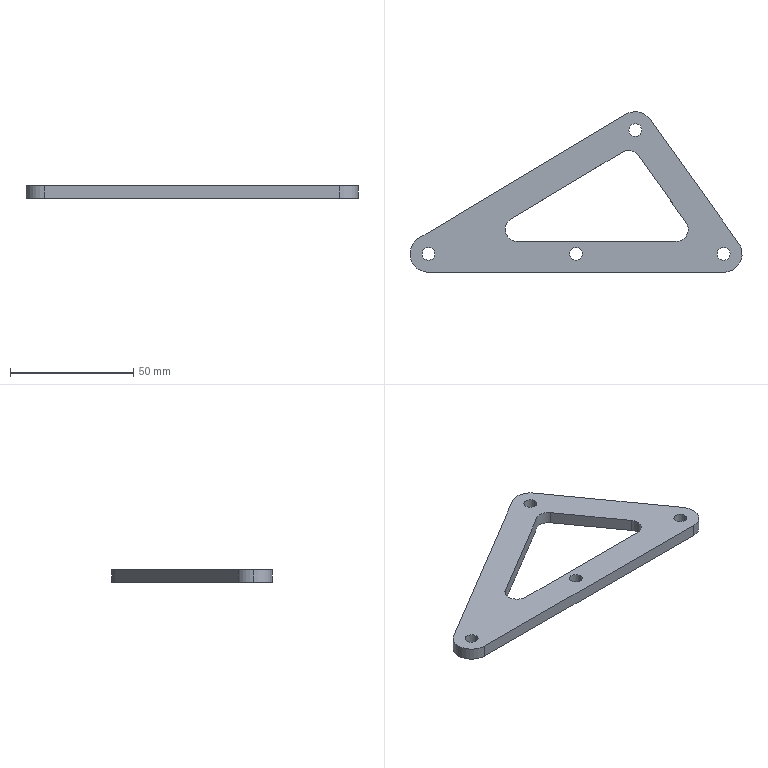Part | SolidWorks | features Extrusion 1 | 1 solid | 24 faces | box 135 x 65.308 x 5 mm | volume 17553 mm3 | cylinder 16 | plane 8 | commonest cylinder face diameters 5.2 x8 10 x4 15 x4
STEP:
#1=CARTESIAN_POINT('',(-50.457,-36.017,5.));
#2=VERTEX_POINT('',#1);
#3=CARTESIAN_POINT('',(-52.89,-40.308,5.));
#4=VERTEX_POINT('',#3);
#5=CARTESIAN_POINT('',(-47.89,-40.308,5.));
#6=DIRECTION('',(0.,0.,1.));
#7=DIRECTION('',(-1.,0.,0.));
#8=AXIS2_PLACEMENT_3D('',#5,#6,#7);
#9=CIRCLE('',#8,5.);
#10=EDGE_CURVE('',#2,#4,#9,.T.);
#11=ORIENTED_EDGE('',*,*,#10,.T.);
#12=CARTESIAN_POINT('',(-52.89,-40.308,0.));
#13=VERTEX_POINT('',#12);
#14=CARTESIAN_POINT('',(-52.89,-40.308,5.));
#15=DIRECTION('',(0.,0.,-1.));
#16=VECTOR('',#15,1000.);
#17=LINE('',#14,#16);
#18=EDGE_CURVE('',#4,#13,#17,.T.);
#19=ORIENTED_EDGE('',*,*,#18,.T.);
#20=CARTESIAN_POINT('',(-50.457,-36.017,0.));
#21=VERTEX_POINT('',#20);
#22=CARTESIAN_POINT('',(-47.89,-40.308,0.));
#23=DIRECTION('',(0.,0.,1.));
#24=DIRECTION('',(-1.,0.,0.));
#25=AXIS2_PLACEMENT_3D('',#22,#23,#24);
#26=CIRCLE('',#25,5.);
#27=EDGE_CURVE('',#21,#13,#26,.T.);
#28=ORIENTED_EDGE('',*,*,#27,.F.);
#29=CARTESIAN_POINT('',(-50.457,-36.017,5.));
#30=DIRECTION('',(0.,0.,-1.));
#31=VECTOR('',#30,1000.);
#32=LINE('',#29,#31);
#33=EDGE_CURVE('',#2,#21,#32,.T.);
#34=ORIENTED_EDGE('',*,*,#33,.F.);
#35=EDGE_LOOP('',(#11,#19,#28,#34));
#36=FACE_OUTER_BOUND('',#35,.T.);
#37=CARTESIAN_POINT('',(-47.89,-40.308,5.));
#38=DIRECTION('',(0.,0.,-1.));
#39=DIRECTION('',(-1.,0.,0.));
#40=AXIS2_PLACEMENT_3D('',#37,#38,#39);
#41=CYLINDRICAL_SURFACE('',#40,5.);
#42=ADVANCED_FACE('',(#36),#41,.F.);
#43=CARTESIAN_POINT('',(-2.6,0.,5.));
#44=VERTEX_POINT('',#43);
#45=CARTESIAN_POINT('',(2.6,0.,5.));
#46=VERTEX_POINT('',#45);
#47=CARTESIAN_POINT('',(0.,0.,5.));
#48=DIRECTION('',(0.,0.,1.));
#49=DIRECTION('',(1.,0.,0.));
#50=AXIS2_PLACEMENT_3D('',#47,#48,#49);
#51=CIRCLE('',#50,2.6);
#52=EDGE_CURVE('',#44,#46,#51,.T.);
#53=ORIENTED_EDGE('',*,*,#52,.T.);
#54=CARTESIAN_POINT('',(2.6,0.,0.));
#55=VERTEX_POINT('',#54);
#56=CARTESIAN_POINT('',(2.6,0.,5.));
#57=DIRECTION('',(0.,0.,-1.));
#58=VECTOR('',#57,1000.);
#59=LINE('',#56,#58);
#60=EDGE_CURVE('',#46,#55,#59,.T.);
#61=ORIENTED_EDGE('',*,*,#60,.T.);
#62=CARTESIAN_POINT('',(-2.6,0.,0.));
#63=VERTEX_POINT('',#62);
#64=CARTESIAN_POINT('',(0.,0.,0.));
#65=DIRECTION('',(0.,0.,1.));
#66=DIRECTION('',(1.,0.,0.));
#67=AXIS2_PLACEMENT_3D('',#64,#65,#66);
#68=CIRCLE('',#67,2.6);
#69=EDGE_CURVE('',#63,#55,#68,.T.);
#70=ORIENTED_EDGE('',*,*,#69,.F.);
#71=CARTESIAN_POINT('',(-2.6,0.,5.));
#72=DIRECTION('',(0.,0.,-1.));
#73=VECTOR('',#72,1000.);
#74=LINE('',#71,#73);
#75=EDGE_CURVE('',#44,#63,#74,.T.);
#76=ORIENTED_EDGE('',*,*,#75,.F.);
#77=EDGE_LOOP('',(#53,#61,#70,#76));
#78=FACE_OUTER_BOUND('',#77,.T.);
#79=CARTESIAN_POINT('',(0.,0.,5.));
#80=DIRECTION('',(0.,0.,-1.));
#81=DIRECTION('',(-1.,0.,0.));
#82=AXIS2_PLACEMENT_3D('',#79,#80,#81);
#83=CYLINDRICAL_SURFACE('',#82,2.6);
#84=ADVANCED_FACE('',(#78),#83,.F.);
#85=CARTESIAN_POINT('',(-86.68,-50.308,5.));
#86=VERTEX_POINT('',#85);
#87=CARTESIAN_POINT('',(-81.48,-50.308,5.));
#88=VERTEX_POINT('',#87);
#89=CARTESIAN_POINT('',(-84.08,-50.308,5.));
#90=DIRECTION('',(0.,0.,1.));
#91=DIRECTION('',(1.,0.,0.));
#92=AXIS2_PLACEMENT_3D('',#89,#90,#91);
#93=CIRCLE('',#92,2.6);
#94=EDGE_CURVE('',#86,#88,#93,.T.);
#95=ORIENTED_EDGE('',*,*,#94,.T.);
#96=CARTESIAN_POINT('',(-81.48,-50.308,0.));
#97=VERTEX_POINT('',#96);
#98=CARTESIAN_POINT('',(-81.48,-50.308,5.));
#99=DIRECTION('',(0.,0.,-1.));
#100=VECTOR('',#99,1000.);
#101=LINE('',#98,#100);
#102=EDGE_CURVE('',#88,#97,#101,.T.);
#103=ORIENTED_EDGE('',*,*,#102,.T.);
#104=CARTESIAN_POINT('',(-86.68,-50.308,0.));
#105=VERTEX_POINT('',#104);
#106=CARTESIAN_POINT('',(-84.08,-50.308,0.));
#107=DIRECTION('',(0.,0.,1.));
#108=DIRECTION('',(1.,0.,0.));
#109=AXIS2_PLACEMENT_3D('',#106,#107,#108);
#110=CIRCLE('',#109,2.6);
#111=EDGE_CURVE('',#105,#97,#110,.T.);
#112=ORIENTED_EDGE('',*,*,#111,.F.);
#113=CARTESIAN_POINT('',(-86.68,-50.308,5.));
#114=DIRECTION('',(0.,0.,-1.));
#115=VECTOR('',#114,1000.);
#116=LINE('',#113,#115);
#117=EDGE_CURVE('',#86,#105,#116,.T.);
#118=ORIENTED_EDGE('',*,*,#117,.F.);
#119=EDGE_LOOP('',(#95,#103,#112,#118));
#120=FACE_OUTER_BOUND('',#119,.T.);
#121=CARTESIAN_POINT('',(-84.08,-50.308,5.));
#122=DIRECTION('',(0.,0.,-1.));
#123=DIRECTION('',(-1.,0.,0.));
#124=AXIS2_PLACEMENT_3D('',#121,#122,#123);
#125=CYLINDRICAL_SURFACE('',#124,2.6);
#126=ADVANCED_FACE('',(#120),#125,.F.);
#127=CARTESIAN_POINT('',(33.32,-50.308,5.));
#128=VERTEX_POINT('',#127);
#129=CARTESIAN_POINT('',(38.52,-50.308,5.));
#130=VERTEX_POINT('',#129);
#131=CARTESIAN_POINT('',(35.92,-50.308,5.));
#132=DIRECTION('',(0.,0.,1.));
#133=DIRECTION('',(1.,0.,0.));
#134=AXIS2_PLACEMENT_3D('',#131,#132,#133);
#135=CIRCLE('',#134,2.6);
#136=EDGE_CURVE('',#128,#130,#135,.T.);
#137=ORIENTED_EDGE('',*,*,#136,.T.);
#138=CARTESIAN_POINT('',(38.52,-50.308,0.));
#139=VERTEX_POINT('',#138);
#140=CARTESIAN_POINT('',(38.52,-50.308,5.));
#141=DIRECTION('',(0.,0.,-1.));
#142=VECTOR('',#141,1000.);
#143=LINE('',#140,#142);
#144=EDGE_CURVE('',#130,#139,#143,.T.);
#145=ORIENTED_EDGE('',*,*,#144,.T.);
#146=CARTESIAN_POINT('',(33.32,-50.308,0.));
#147=VERTEX_POINT('',#146);
#148=CARTESIAN_POINT('',(35.92,-50.308,0.));
#149=DIRECTION('',(0.,0.,1.));
#150=DIRECTION('',(1.,0.,0.));
#151=AXIS2_PLACEMENT_3D('',#148,#149,#150);
#152=CIRCLE('',#151,2.6);
#153=EDGE_CURVE('',#147,#139,#152,.T.);
#154=ORIENTED_EDGE('',*,*,#153,.F.);
#155=CARTESIAN_POINT('',(33.32,-50.308,5.));
#156=DIRECTION('',(0.,0.,-1.));
#157=VECTOR('',#156,1000.);
#158=LINE('',#155,#157);
#159=EDGE_CURVE('',#128,#147,#158,.T.);
#160=ORIENTED_EDGE('',*,*,#159,.F.);
#161=EDGE_LOOP('',(#137,#145,#154,#160));
#162=FACE_OUTER_BOUND('',#161,.T.);
#163=CARTESIAN_POINT('',(35.92,-50.308,5.));
#164=DIRECTION('',(0.,0.,-1.));
#165=DIRECTION('',(-1.,0.,0.));
#166=AXIS2_PLACEMENT_3D('',#163,#164,#165);
#167=CYLINDRICAL_SURFACE('',#166,2.6);
#168=ADVANCED_FACE('',(#162),#167,.F.);
#169=CARTESIAN_POINT('',(-26.68,-50.308,5.));
#170=VERTEX_POINT('',#169);
#171=CARTESIAN_POINT('',(-21.48,-50.308,5.));
#172=VERTEX_POINT('',#171);
#173=CARTESIAN_POINT('',(-24.08,-50.308,5.));
#174=DIRECTION('',(0.,0.,1.));
#175=DIRECTION('',(1.,0.,0.));
#176=AXIS2_PLACEMENT_3D('',#173,#174,#175);
#177=CIRCLE('',#176,2.6);
#178=EDGE_CURVE('',#170,#172,#177,.T.);
#179=ORIENTED_EDGE('',*,*,#178,.T.);
#180=CARTESIAN_POINT('',(-21.48,-50.308,0.));
#181=VERTEX_POINT('',#180);
#182=CARTESIAN_POINT('',(-21.48,-50.308,5.));
#183=DIRECTION('',(0.,0.,-1.));
#184=VECTOR('',#183,1000.);
#185=LINE('',#182,#184);
#186=EDGE_CURVE('',#172,#181,#185,.T.);
#187=ORIENTED_EDGE('',*,*,#186,.T.);
#188=CARTESIAN_POINT('',(-26.68,-50.308,0.));
#189=VERTEX_POINT('',#188);
#190=CARTESIAN_POINT('',(-24.08,-50.308,0.));
#191=DIRECTION('',(0.,0.,1.));
#192=DIRECTION('',(1.,0.,0.));
#193=AXIS2_PLACEMENT_3D('',#190,#191,#192);
#194=CIRCLE('',#193,2.6);
#195=EDGE_CURVE('',#189,#181,#194,.T.);
#196=ORIENTED_EDGE('',*,*,#195,.F.);
#197=CARTESIAN_POINT('',(-26.68,-50.308,5.));
#198=DIRECTION('',(0.,0.,-1.));
#199=VECTOR('',#198,1000.);
#200=LINE('',#197,#199);
#201=EDGE_CURVE('',#170,#189,#200,.T.);
#202=ORIENTED_EDGE('',*,*,#201,.F.);
#203=EDGE_LOOP('',(#179,#187,#196,#202));
#204=FACE_OUTER_BOUND('',#203,.T.);
#205=CARTESIAN_POINT('',(-24.08,-50.308,5.));
#206=DIRECTION('',(0.,0.,-1.));
#207=DIRECTION('',(-1.,0.,0.));
#208=AXIS2_PLACEMENT_3D('',#205,#206,#207);
#209=CYLINDRICAL_SURFACE('',#208,2.6);
#210=ADVANCED_FACE('',(#204),#209,.F.);
#211=CARTESIAN_POINT('',(-91.58,-50.308,5.));
#212=VERTEX_POINT('',#211);
#213=CARTESIAN_POINT('',(-84.08,-57.808,5.));
#214=VERTEX_POINT('',#213);
#215=CARTESIAN_POINT('',(-84.08,-50.308,5.));
#216=DIRECTION('',(0.,0.,1.));
#217=DIRECTION('',(1.,0.,0.));
#218=AXIS2_PLACEMENT_3D('',#215,#216,#217);
#219=CIRCLE('',#218,7.5);
#220=EDGE_CURVE('',#212,#214,#219,.T.);
#221=ORIENTED_EDGE('',*,*,#220,.F.);
#222=CARTESIAN_POINT('',(-91.58,-50.308,0.));
#223=VERTEX_POINT('',#222);
#224=CARTESIAN_POINT('',(-91.58,-50.308,5.));
#225=DIRECTION('',(0.,0.,-1.));
#226=VECTOR('',#225,1000.);
#227=LINE('',#224,#226);
#228=EDGE_CURVE('',#212,#223,#227,.T.);
#229=ORIENTED_EDGE('',*,*,#228,.T.);
#230=CARTESIAN_POINT('',(-84.08,-57.808,0.));
#231=VERTEX_POINT('',#230);
#232=CARTESIAN_POINT('',(-84.08,-50.308,0.));
#233=DIRECTION('',(0.,0.,1.));
#234=DIRECTION('',(1.,0.,0.));
#235=AXIS2_PLACEMENT_3D('',#232,#233,#234);
#236=CIRCLE('',#235,7.5);
#237=EDGE_CURVE('',#223,#231,#236,.T.);
#238=ORIENTED_EDGE('',*,*,#237,.T.);
#239=CARTESIAN_POINT('',(-84.08,-57.808,5.));
#240=DIRECTION('',(0.,0.,-1.));
#241=VECTOR('',#240,1000.);
#242=LINE('',#239,#241);
#243=EDGE_CURVE('',#214,#231,#242,.T.);
#244=ORIENTED_EDGE('',*,*,#243,.F.);
#245=EDGE_LOOP('',(#221,#229,#238,#244));
#246=FACE_OUTER_BOUND('',#245,.T.);
#247=CARTESIAN_POINT('',(-84.08,-50.308,5.));
#248=DIRECTION('',(0.,0.,-1.));
#249=DIRECTION('',(-1.,0.,0.));
#250=AXIS2_PLACEMENT_3D('',#247,#248,#249);
#251=CYLINDRICAL_SURFACE('',#250,7.5);
#252=ADVANCED_FACE('',(#246),#251,.T.);
#253=ORIENTED_EDGE('',*,*,#94,.F.);
#254=CARTESIAN_POINT('',(-84.08,-50.308,5.));
#255=DIRECTION('',(0.,0.,1.));
#256=DIRECTION('',(1.,0.,0.));
#257=AXIS2_PLACEMENT_3D('',#254,#255,#256);
#258=CIRCLE('',#257,2.6);
#259=EDGE_CURVE('',#88,#86,#258,.T.);
#260=ORIENTED_EDGE('',*,*,#259,.F.);
#261=EDGE_LOOP('',(#253,#260));
#262=FACE_BOUND('',#261,.T.);
#263=ORIENTED_EDGE('',*,*,#178,.F.);
#264=CARTESIAN_POINT('',(-24.08,-50.308,5.));
#265=DIRECTION('',(0.,0.,1.));
#266=DIRECTION('',(1.,0.,0.));
#267=AXIS2_PLACEMENT_3D('',#264,#265,#266);
#268=CIRCLE('',#267,2.6);
#269=EDGE_CURVE('',#172,#170,#268,.T.);
#270=ORIENTED_EDGE('',*,*,#269,.F.);
#271=EDGE_LOOP('',(#263,#270));
#272=FACE_BOUND('',#271,.T.);
#273=CARTESIAN_POINT('',(35.92,-57.808,5.));
#274=VERTEX_POINT('',#273);
#275=CARTESIAN_POINT('',(-24.08,-57.808,5.));
#276=DIRECTION('',(1.,0.,0.));
#277=VECTOR('',#276,1000.);
#278=LINE('',#275,#277);
#279=EDGE_CURVE('',#214,#274,#278,.T.);
#280=ORIENTED_EDGE('',*,*,#279,.T.);
#281=CARTESIAN_POINT('',(42.024,-45.949,5.));
#282=VERTEX_POINT('',#281);
#283=CARTESIAN_POINT('',(35.92,-50.308,5.));
#284=DIRECTION('',(0.,0.,1.));
#285=DIRECTION('',(1.,0.,0.));
#286=AXIS2_PLACEMENT_3D('',#283,#284,#285);
#287=CIRCLE('',#286,7.5);
#288=EDGE_CURVE('',#274,#282,#287,.T.);
#289=ORIENTED_EDGE('',*,*,#288,.T.);
#290=CARTESIAN_POINT('',(6.104,4.358,5.));
#291=VERTEX_POINT('',#290);
#292=CARTESIAN_POINT('',(42.024,-45.949,5.));
#293=DIRECTION('',(-0.5811,0.8138,0.));
#294=VECTOR('',#293,1000.);
#295=LINE('',#292,#294);
#296=EDGE_CURVE('',#282,#291,#295,.T.);
#297=ORIENTED_EDGE('',*,*,#296,.T.);
#298=CARTESIAN_POINT('',(-3.851,6.436,5.));
#299=VERTEX_POINT('',#298);
#300=CARTESIAN_POINT('',(0.,0.,5.));
#301=DIRECTION('',(0.,0.,1.));
#302=DIRECTION('',(1.,0.,0.));
#303=AXIS2_PLACEMENT_3D('',#300,#301,#302);
#304=CIRCLE('',#303,7.5);
#305=EDGE_CURVE('',#291,#299,#304,.T.);
#306=ORIENTED_EDGE('',*,*,#305,.T.);
#307=CARTESIAN_POINT('',(-87.93,-43.872,5.));
#308=VERTEX_POINT('',#307);
#309=CARTESIAN_POINT('',(-3.851,6.436,5.));
#310=DIRECTION('',(-0.8581,-0.5134,0.));
#311=VECTOR('',#310,1000.);
#312=LINE('',#309,#311);
#313=EDGE_CURVE('',#299,#308,#312,.T.);
#314=ORIENTED_EDGE('',*,*,#313,.T.);
#315=CARTESIAN_POINT('',(-84.08,-50.308,5.));
#316=DIRECTION('',(0.,0.,1.));
#317=DIRECTION('',(1.,0.,0.));
#318=AXIS2_PLACEMENT_3D('',#315,#316,#317);
#319=CIRCLE('',#318,7.5);
#320=EDGE_CURVE('',#308,#212,#319,.T.);
#321=ORIENTED_EDGE('',*,*,#320,.T.);
#322=ORIENTED_EDGE('',*,*,#220,.T.);
#323=EDGE_LOOP('',(#280,#289,#297,#306,#314,#321,#322));
#324=FACE_OUTER_BOUND('',#323,.T.);
#325=ORIENTED_EDGE('',*,*,#136,.F.);
#326=CARTESIAN_POINT('',(35.92,-50.308,5.));
#327=DIRECTION('',(0.,0.,1.));
#328=DIRECTION('',(1.,0.,0.));
#329=AXIS2_PLACEMENT_3D('',#326,#327,#328);
#330=CIRCLE('',#329,2.6);
#331=EDGE_CURVE('',#130,#128,#330,.T.);
#332=ORIENTED_EDGE('',*,*,#331,.F.);
#333=EDGE_LOOP('',(#325,#332));
#334=FACE_BOUND('',#333,.T.);
#335=ORIENTED_EDGE('',*,*,#52,.F.);
#336=CARTESIAN_POINT('',(0.,0.,5.));
#337=DIRECTION('',(0.,0.,1.));
#338=DIRECTION('',(1.,0.,0.));
#339=AXIS2_PLACEMENT_3D('',#336,#337,#338);
#340=CIRCLE('',#339,2.6);
#341=EDGE_CURVE('',#46,#44,#340,.T.);
#342=ORIENTED_EDGE('',*,*,#341,.F.);
#343=EDGE_LOOP('',(#335,#342));
#344=FACE_BOUND('',#343,.T.);
#345=CARTESIAN_POINT('',(20.562,-37.402,5.));
#346=VERTEX_POINT('',#345);
#347=CARTESIAN_POINT('',(1.29,-10.411,5.));
#348=VERTEX_POINT('',#347);
#349=CARTESIAN_POINT('',(20.562,-37.402,5.));
#350=DIRECTION('',(-0.5811,0.8138,0.));
#351=VECTOR('',#350,1000.);
#352=LINE('',#349,#351);
#353=EDGE_CURVE('',#346,#348,#352,.T.);
#354=ORIENTED_EDGE('',*,*,#353,.F.);
#355=CARTESIAN_POINT('',(16.493,-45.308,5.));
#356=VERTEX_POINT('',#355);
#357=CARTESIAN_POINT('',(16.493,-40.308,5.));
#358=DIRECTION('',(0.,0.,1.));
#359=DIRECTION('',(1.,0.,0.));
#360=AXIS2_PLACEMENT_3D('',#357,#358,#359);
#361=CIRCLE('',#360,5.);
#362=EDGE_CURVE('',#356,#346,#361,.T.);
#363=ORIENTED_EDGE('',*,*,#362,.F.);
#364=CARTESIAN_POINT('',(-47.89,-45.308,5.));
#365=VERTEX_POINT('',#364);
#366=CARTESIAN_POINT('',(-24.08,-45.308,5.));
#367=DIRECTION('',(1.,0.,0.));
#368=VECTOR('',#367,1000.);
#369=LINE('',#366,#368);
#370=EDGE_CURVE('',#365,#356,#369,.T.);
#371=ORIENTED_EDGE('',*,*,#370,.F.);
#372=CARTESIAN_POINT('',(-47.89,-40.308,5.));
#373=DIRECTION('',(0.,0.,1.));
#374=DIRECTION('',(-1.,0.,0.));
#375=AXIS2_PLACEMENT_3D('',#372,#373,#374);
#376=CIRCLE('',#375,5.);
#377=EDGE_CURVE('',#4,#365,#376,.T.);
#378=ORIENTED_EDGE('',*,*,#377,.F.);
#379=ORIENTED_EDGE('',*,*,#10,.F.);
#380=CARTESIAN_POINT('',(-5.347,-9.026,5.));
#381=VERTEX_POINT('',#380);
#382=CARTESIAN_POINT('',(-5.347,-9.026,5.));
#383=DIRECTION('',(-0.8581,-0.5134,0.));
#384=VECTOR('',#383,1000.);
#385=LINE('',#382,#384);
#386=EDGE_CURVE('',#381,#2,#385,.T.);
#387=ORIENTED_EDGE('',*,*,#386,.F.);
#388=CARTESIAN_POINT('',(-2.779,-13.316,5.));
#389=DIRECTION('',(0.,0.,1.));
#390=DIRECTION('',(1.,0.,0.));
#391=AXIS2_PLACEMENT_3D('',#388,#389,#390);
#392=CIRCLE('',#391,5.);
#393=EDGE_CURVE('',#348,#381,#392,.T.);
#394=ORIENTED_EDGE('',*,*,#393,.F.);
#395=EDGE_LOOP('',(#354,#363,#371,#378,#379,#387,#394));
#396=FACE_BOUND('',#395,.T.);
#397=CARTESIAN_POINT('',(35.92,-50.308,5.));
#398=DIRECTION('',(0.,0.,1.));
#399=DIRECTION('',(1.,0.,0.));
#400=AXIS2_PLACEMENT_3D('',#397,#398,#399);
#401=PLANE('',#400);
#402=ADVANCED_FACE('',(#262,#272,#324,#334,#344,#396),#401,.T.);
#403=ORIENTED_EDGE('',*,*,#69,.T.);
#404=CARTESIAN_POINT('',(0.,0.,0.));
#405=DIRECTION('',(0.,0.,1.));
#406=DIRECTION('',(1.,0.,0.));
#407=AXIS2_PLACEMENT_3D('',#404,#405,#406);
#408=CIRCLE('',#407,2.6);
#409=EDGE_CURVE('',#55,#63,#408,.T.);
#410=ORIENTED_EDGE('',*,*,#409,.T.);
#411=EDGE_LOOP('',(#403,#410));
#412=FACE_BOUND('',#411,.T.);
#413=ORIENTED_EDGE('',*,*,#111,.T.);
#414=CARTESIAN_POINT('',(-84.08,-50.308,0.));
#415=DIRECTION('',(0.,0.,1.));
#416=DIRECTION('',(1.,0.,0.));
#417=AXIS2_PLACEMENT_3D('',#414,#415,#416);
#418=CIRCLE('',#417,2.6);
#419=EDGE_CURVE('',#97,#105,#418,.T.);
#420=ORIENTED_EDGE('',*,*,#419,.T.);
#421=EDGE_LOOP('',(#413,#420));
#422=FACE_BOUND('',#421,.T.);
#423=ORIENTED_EDGE('',*,*,#153,.T.);
#424=CARTESIAN_POINT('',(35.92,-50.308,0.));
#425=DIRECTION('',(0.,0.,1.));
#426=DIRECTION('',(1.,0.,0.));
#427=AXIS2_PLACEMENT_3D('',#424,#425,#426);
#428=CIRCLE('',#427,2.6);
#429=EDGE_CURVE('',#139,#147,#428,.T.);
#430=ORIENTED_EDGE('',*,*,#429,.T.);
#431=EDGE_LOOP('',(#423,#430));
#432=FACE_BOUND('',#431,.T.);
#433=ORIENTED_EDGE('',*,*,#195,.T.);
#434=CARTESIAN_POINT('',(-24.08,-50.308,0.));
#435=DIRECTION('',(0.,0.,1.));
#436=DIRECTION('',(1.,0.,0.));
#437=AXIS2_PLACEMENT_3D('',#434,#435,#436);
#438=CIRCLE('',#437,2.6);
#439=EDGE_CURVE('',#181,#189,#438,.T.);
#440=ORIENTED_EDGE('',*,*,#439,.T.);
#441=EDGE_LOOP('',(#433,#440));
#442=FACE_BOUND('',#441,.T.);
#443=CARTESIAN_POINT('',(35.92,-57.808,0.));
#444=VERTEX_POINT('',#443);
#445=CARTESIAN_POINT('',(42.024,-45.949,0.));
#446=VERTEX_POINT('',#445);
#447=CARTESIAN_POINT('',(35.92,-50.308,0.));
#448=DIRECTION('',(0.,0.,1.));
#449=DIRECTION('',(1.,0.,0.));
#450=AXIS2_PLACEMENT_3D('',#447,#448,#449);
#451=CIRCLE('',#450,7.5);
#452=EDGE_CURVE('',#444,#446,#451,.T.);
#453=ORIENTED_EDGE('',*,*,#452,.F.);
#454=CARTESIAN_POINT('',(-84.08,-57.808,0.));
#455=DIRECTION('',(1.,0.,0.));
#456=VECTOR('',#455,1000.);
#457=LINE('',#454,#456);
#458=EDGE_CURVE('',#231,#444,#457,.T.);
#459=ORIENTED_EDGE('',*,*,#458,.F.);
#460=ORIENTED_EDGE('',*,*,#237,.F.);
#461=CARTESIAN_POINT('',(-87.93,-43.872,0.));
#462=VERTEX_POINT('',#461);
#463=CARTESIAN_POINT('',(-84.08,-50.308,0.));
#464=DIRECTION('',(0.,0.,1.));
#465=DIRECTION('',(1.,0.,0.));
#466=AXIS2_PLACEMENT_3D('',#463,#464,#465);
#467=CIRCLE('',#466,7.5);
#468=EDGE_CURVE('',#462,#223,#467,.T.);
#469=ORIENTED_EDGE('',*,*,#468,.F.);
#470=CARTESIAN_POINT('',(-3.851,6.436,0.));
#471=VERTEX_POINT('',#470);
#472=CARTESIAN_POINT('',(-3.851,6.436,0.));
#473=DIRECTION('',(-0.8581,-0.5134,0.));
#474=VECTOR('',#473,1000.);
#475=LINE('',#472,#474);
#476=EDGE_CURVE('',#471,#462,#475,.T.);
#477=ORIENTED_EDGE('',*,*,#476,.F.);
#478=CARTESIAN_POINT('',(6.104,4.358,0.));
#479=VERTEX_POINT('',#478);
#480=CARTESIAN_POINT('',(0.,0.,0.));
#481=DIRECTION('',(0.,0.,1.));
#482=DIRECTION('',(1.,0.,0.));
#483=AXIS2_PLACEMENT_3D('',#480,#481,#482);
#484=CIRCLE('',#483,7.5);
#485=EDGE_CURVE('',#479,#471,#484,.T.);
#486=ORIENTED_EDGE('',*,*,#485,.F.);
#487=CARTESIAN_POINT('',(42.024,-45.949,0.));
#488=DIRECTION('',(-0.5811,0.8138,0.));
#489=VECTOR('',#488,1000.);
#490=LINE('',#487,#489);
#491=EDGE_CURVE('',#446,#479,#490,.T.);
#492=ORIENTED_EDGE('',*,*,#491,.F.);
#493=EDGE_LOOP('',(#453,#459,#460,#469,#477,#486,#492));
#494=FACE_OUTER_BOUND('',#493,.T.);
#495=CARTESIAN_POINT('',(16.493,-45.308,0.));
#496=VERTEX_POINT('',#495);
#497=CARTESIAN_POINT('',(20.562,-37.402,0.));
#498=VERTEX_POINT('',#497);
#499=CARTESIAN_POINT('',(16.493,-40.308,0.));
#500=DIRECTION('',(0.,0.,1.));
#501=DIRECTION('',(1.,0.,0.));
#502=AXIS2_PLACEMENT_3D('',#499,#500,#501);
#503=CIRCLE('',#502,5.);
#504=EDGE_CURVE('',#496,#498,#503,.T.);
#505=ORIENTED_EDGE('',*,*,#504,.T.);
#506=CARTESIAN_POINT('',(1.29,-10.411,0.));
#507=VERTEX_POINT('',#506);
#508=CARTESIAN_POINT('',(20.562,-37.402,0.));
#509=DIRECTION('',(-0.5811,0.8138,0.));
#510=VECTOR('',#509,1000.);
#511=LINE('',#508,#510);
#512=EDGE_CURVE('',#498,#507,#511,.T.);
#513=ORIENTED_EDGE('',*,*,#512,.T.);
#514=CARTESIAN_POINT('',(-5.347,-9.026,0.));
#515=VERTEX_POINT('',#514);
#516=CARTESIAN_POINT('',(-2.779,-13.316,0.));
#517=DIRECTION('',(0.,0.,1.));
#518=DIRECTION('',(1.,0.,0.));
#519=AXIS2_PLACEMENT_3D('',#516,#517,#518);
#520=CIRCLE('',#519,5.);
#521=EDGE_CURVE('',#507,#515,#520,.T.);
#522=ORIENTED_EDGE('',*,*,#521,.T.);
#523=CARTESIAN_POINT('',(-5.347,-9.026,0.));
#524=DIRECTION('',(-0.8581,-0.5134,0.));
#525=VECTOR('',#524,1000.);
#526=LINE('',#523,#525);
#527=EDGE_CURVE('',#515,#21,#526,.T.);
#528=ORIENTED_EDGE('',*,*,#527,.T.);
#529=ORIENTED_EDGE('',*,*,#27,.T.);
#530=CARTESIAN_POINT('',(-47.89,-45.308,0.));
#531=VERTEX_POINT('',#530);
#532=CARTESIAN_POINT('',(-47.89,-40.308,0.));
#533=DIRECTION('',(0.,0.,1.));
#534=DIRECTION('',(-1.,0.,0.));
#535=AXIS2_PLACEMENT_3D('',#532,#533,#534);
#536=CIRCLE('',#535,5.);
#537=EDGE_CURVE('',#13,#531,#536,.T.);
#538=ORIENTED_EDGE('',*,*,#537,.T.);
#539=CARTESIAN_POINT('',(-47.89,-45.308,0.));
#540=DIRECTION('',(1.,0.,0.));
#541=VECTOR('',#540,1000.);
#542=LINE('',#539,#541);
#543=EDGE_CURVE('',#531,#496,#542,.T.);
#544=ORIENTED_EDGE('',*,*,#543,.T.);
#545=EDGE_LOOP('',(#505,#513,#522,#528,#529,#538,#544));
#546=FACE_BOUND('',#545,.T.);
#547=CARTESIAN_POINT('',(35.92,-50.308,0.));
#548=DIRECTION('',(0.,0.,1.));
#549=DIRECTION('',(1.,0.,0.));
#550=AXIS2_PLACEMENT_3D('',#547,#548,#549);
#551=PLANE('',#550);
#552=ADVANCED_FACE('',(#412,#422,#432,#442,#494,#546),#551,.F.);
#553=ORIENTED_EDGE('',*,*,#452,.T.);
#554=CARTESIAN_POINT('',(42.024,-45.949,5.));
#555=DIRECTION('',(0.,0.,-1.));
#556=VECTOR('',#555,1000.);
#557=LINE('',#554,#556);
#558=EDGE_CURVE('',#282,#446,#557,.T.);
#559=ORIENTED_EDGE('',*,*,#558,.F.);
#560=ORIENTED_EDGE('',*,*,#288,.F.);
#561=CARTESIAN_POINT('',(35.92,-57.808,5.));
#562=DIRECTION('',(0.,0.,-1.));
#563=VECTOR('',#562,1000.);
#564=LINE('',#561,#563);
#565=EDGE_CURVE('',#274,#444,#564,.T.);
#566=ORIENTED_EDGE('',*,*,#565,.T.);
#567=EDGE_LOOP('',(#553,#559,#560,#566));
#568=FACE_OUTER_BOUND('',#567,.T.);
#569=CARTESIAN_POINT('',(35.92,-50.308,5.));
#570=DIRECTION('',(0.,0.,-1.));
#571=DIRECTION('',(-1.,0.,0.));
#572=AXIS2_PLACEMENT_3D('',#569,#570,#571);
#573=CYLINDRICAL_SURFACE('',#572,7.5);
#574=ADVANCED_FACE('',(#568),#573,.T.);
#575=ORIENTED_EDGE('',*,*,#491,.T.);
#576=CARTESIAN_POINT('',(6.104,4.358,5.));
#577=DIRECTION('',(0.,0.,-1.));
#578=VECTOR('',#577,1000.);
#579=LINE('',#576,#578);
#580=EDGE_CURVE('',#291,#479,#579,.T.);
#581=ORIENTED_EDGE('',*,*,#580,.F.);
#582=ORIENTED_EDGE('',*,*,#296,.F.);
#583=ORIENTED_EDGE('',*,*,#558,.T.);
#584=EDGE_LOOP('',(#575,#581,#582,#583));
#585=FACE_OUTER_BOUND('',#584,.T.);
#586=CARTESIAN_POINT('',(42.024,-45.949,5.));
#587=DIRECTION('',(-0.8138,-0.5811,0.));
#588=DIRECTION('',(0.5811,-0.8138,0.));
#589=AXIS2_PLACEMENT_3D('',#586,#587,#588);
#590=PLANE('',#589);
#591=ADVANCED_FACE('',(#585),#590,.F.);
#592=ORIENTED_EDGE('',*,*,#485,.T.);
#593=CARTESIAN_POINT('',(-3.851,6.436,5.));
#594=DIRECTION('',(0.,0.,-1.));
#595=VECTOR('',#594,1000.);
#596=LINE('',#593,#595);
#597=EDGE_CURVE('',#299,#471,#596,.T.);
#598=ORIENTED_EDGE('',*,*,#597,.F.);
#599=ORIENTED_EDGE('',*,*,#305,.F.);
#600=ORIENTED_EDGE('',*,*,#580,.T.);
#601=EDGE_LOOP('',(#592,#598,#599,#600));
#602=FACE_OUTER_BOUND('',#601,.T.);
#603=CARTESIAN_POINT('',(0.,0.,5.));
#604=DIRECTION('',(0.,0.,-1.));
#605=DIRECTION('',(-1.,0.,0.));
#606=AXIS2_PLACEMENT_3D('',#603,#604,#605);
#607=CYLINDRICAL_SURFACE('',#606,7.5);
#608=ADVANCED_FACE('',(#602),#607,.T.);
#609=ORIENTED_EDGE('',*,*,#476,.T.);
#610=CARTESIAN_POINT('',(-87.93,-43.872,5.));
#611=DIRECTION('',(0.,0.,-1.));
#612=VECTOR('',#611,1000.);
#613=LINE('',#610,#612);
#614=EDGE_CURVE('',#308,#462,#613,.T.);
#615=ORIENTED_EDGE('',*,*,#614,.F.);
#616=ORIENTED_EDGE('',*,*,#313,.F.);
#617=ORIENTED_EDGE('',*,*,#597,.T.);
#618=EDGE_LOOP('',(#609,#615,#616,#617));
#619=FACE_OUTER_BOUND('',#618,.T.);
#620=CARTESIAN_POINT('',(-3.851,6.436,5.));
#621=DIRECTION('',(0.5134,-0.8581,0.));
#622=DIRECTION('',(0.8581,0.5134,0.));
#623=AXIS2_PLACEMENT_3D('',#620,#621,#622);
#624=PLANE('',#623);
#625=ADVANCED_FACE('',(#619),#624,.F.);
#626=ORIENTED_EDGE('',*,*,#228,.F.);
#627=ORIENTED_EDGE('',*,*,#320,.F.);
#628=ORIENTED_EDGE('',*,*,#614,.T.);
#629=ORIENTED_EDGE('',*,*,#468,.T.);
#630=EDGE_LOOP('',(#626,#627,#628,#629));
#631=FACE_OUTER_BOUND('',#630,.T.);
#632=CARTESIAN_POINT('',(-84.08,-50.308,5.));
#633=DIRECTION('',(0.,0.,-1.));
#634=DIRECTION('',(-1.,0.,0.));
#635=AXIS2_PLACEMENT_3D('',#632,#633,#634);
#636=CYLINDRICAL_SURFACE('',#635,7.5);
#637=ADVANCED_FACE('',(#631),#636,.T.);
#638=ORIENTED_EDGE('',*,*,#458,.T.);
#639=ORIENTED_EDGE('',*,*,#565,.F.);
#640=ORIENTED_EDGE('',*,*,#279,.F.);
#641=ORIENTED_EDGE('',*,*,#243,.T.);
#642=EDGE_LOOP('',(#638,#639,#640,#641));
#643=FACE_OUTER_BOUND('',#642,.T.);
#644=CARTESIAN_POINT('',(-84.08,-57.808,5.));
#645=DIRECTION('',(0.,1.,0.));
#646=DIRECTION('',(0.,0.,1.));
#647=AXIS2_PLACEMENT_3D('',#644,#645,#646);
#648=PLANE('',#647);
#649=ADVANCED_FACE('',(#643),#648,.F.);
#650=ORIENTED_EDGE('',*,*,#186,.F.);
#651=ORIENTED_EDGE('',*,*,#269,.T.);
#652=ORIENTED_EDGE('',*,*,#201,.T.);
#653=ORIENTED_EDGE('',*,*,#439,.F.);
#654=EDGE_LOOP('',(#650,#651,#652,#653));
#655=FACE_OUTER_BOUND('',#654,.T.);
#656=CARTESIAN_POINT('',(-24.08,-50.308,5.));
#657=DIRECTION('',(0.,0.,-1.));
#658=DIRECTION('',(-1.,0.,0.));
#659=AXIS2_PLACEMENT_3D('',#656,#657,#658);
#660=CYLINDRICAL_SURFACE('',#659,2.6);
#661=ADVANCED_FACE('',(#655),#660,.F.);
#662=ORIENTED_EDGE('',*,*,#144,.F.);
#663=ORIENTED_EDGE('',*,*,#331,.T.);
#664=ORIENTED_EDGE('',*,*,#159,.T.);
#665=ORIENTED_EDGE('',*,*,#429,.F.);
#666=EDGE_LOOP('',(#662,#663,#664,#665));
#667=FACE_OUTER_BOUND('',#666,.T.);
#668=CARTESIAN_POINT('',(35.92,-50.308,5.));
#669=DIRECTION('',(0.,0.,-1.));
#670=DIRECTION('',(-1.,0.,0.));
#671=AXIS2_PLACEMENT_3D('',#668,#669,#670);
#672=CYLINDRICAL_SURFACE('',#671,2.6);
#673=ADVANCED_FACE('',(#667),#672,.F.);
#674=ORIENTED_EDGE('',*,*,#102,.F.);
#675=ORIENTED_EDGE('',*,*,#259,.T.);
#676=ORIENTED_EDGE('',*,*,#117,.T.);
#677=ORIENTED_EDGE('',*,*,#419,.F.);
#678=EDGE_LOOP('',(#674,#675,#676,#677));
#679=FACE_OUTER_BOUND('',#678,.T.);
#680=CARTESIAN_POINT('',(-84.08,-50.308,5.));
#681=DIRECTION('',(0.,0.,-1.));
#682=DIRECTION('',(-1.,0.,0.));
#683=AXIS2_PLACEMENT_3D('',#680,#681,#682);
#684=CYLINDRICAL_SURFACE('',#683,2.6);
#685=ADVANCED_FACE('',(#679),#684,.F.);
#686=ORIENTED_EDGE('',*,*,#60,.F.);
#687=ORIENTED_EDGE('',*,*,#341,.T.);
#688=ORIENTED_EDGE('',*,*,#75,.T.);
#689=ORIENTED_EDGE('',*,*,#409,.F.);
#690=EDGE_LOOP('',(#686,#687,#688,#689));
#691=FACE_OUTER_BOUND('',#690,.T.);
#692=CARTESIAN_POINT('',(0.,0.,5.));
#693=DIRECTION('',(0.,0.,-1.));
#694=DIRECTION('',(-1.,0.,0.));
#695=AXIS2_PLACEMENT_3D('',#692,#693,#694);
#696=CYLINDRICAL_SURFACE('',#695,2.6);
#697=ADVANCED_FACE('',(#691),#696,.F.);
#698=ORIENTED_EDGE('',*,*,#504,.F.);
#699=CARTESIAN_POINT('',(16.493,-45.308,5.));
#700=DIRECTION('',(0.,0.,-1.));
#701=VECTOR('',#700,1000.);
#702=LINE('',#699,#701);
#703=EDGE_CURVE('',#356,#496,#702,.T.);
#704=ORIENTED_EDGE('',*,*,#703,.F.);
#705=ORIENTED_EDGE('',*,*,#362,.T.);
#706=CARTESIAN_POINT('',(20.562,-37.402,5.));
#707=DIRECTION('',(0.,0.,-1.));
#708=VECTOR('',#707,1000.);
#709=LINE('',#706,#708);
#710=EDGE_CURVE('',#346,#498,#709,.T.);
#711=ORIENTED_EDGE('',*,*,#710,.T.);
#712=EDGE_LOOP('',(#698,#704,#705,#711));
#713=FACE_OUTER_BOUND('',#712,.T.);
#714=CARTESIAN_POINT('',(16.493,-40.308,5.));
#715=DIRECTION('',(0.,0.,-1.));
#716=DIRECTION('',(-1.,0.,0.));
#717=AXIS2_PLACEMENT_3D('',#714,#715,#716);
#718=CYLINDRICAL_SURFACE('',#717,5.);
#719=ADVANCED_FACE('',(#713),#718,.F.);
#720=ORIENTED_EDGE('',*,*,#512,.F.);
#721=ORIENTED_EDGE('',*,*,#710,.F.);
#722=ORIENTED_EDGE('',*,*,#353,.T.);
#723=CARTESIAN_POINT('',(1.29,-10.411,5.));
#724=DIRECTION('',(0.,0.,-1.));
#725=VECTOR('',#724,1000.);
#726=LINE('',#723,#725);
#727=EDGE_CURVE('',#348,#507,#726,.T.);
#728=ORIENTED_EDGE('',*,*,#727,.T.);
#729=EDGE_LOOP('',(#720,#721,#722,#728));
#730=FACE_OUTER_BOUND('',#729,.T.);
#731=CARTESIAN_POINT('',(20.562,-37.402,5.));
#732=DIRECTION('',(-0.8138,-0.5811,0.));
#733=DIRECTION('',(0.5811,-0.8138,0.));
#734=AXIS2_PLACEMENT_3D('',#731,#732,#733);
#735=PLANE('',#734);
#736=ADVANCED_FACE('',(#730),#735,.T.);
#737=ORIENTED_EDGE('',*,*,#521,.F.);
#738=ORIENTED_EDGE('',*,*,#727,.F.);
#739=ORIENTED_EDGE('',*,*,#393,.T.);
#740=CARTESIAN_POINT('',(-5.347,-9.026,5.));
#741=DIRECTION('',(0.,0.,-1.));
#742=VECTOR('',#741,1000.);
#743=LINE('',#740,#742);
#744=EDGE_CURVE('',#381,#515,#743,.T.);
#745=ORIENTED_EDGE('',*,*,#744,.T.);
#746=EDGE_LOOP('',(#737,#738,#739,#745));
#747=FACE_OUTER_BOUND('',#746,.T.);
#748=CARTESIAN_POINT('',(-2.779,-13.316,5.));
#749=DIRECTION('',(0.,0.,-1.));
#750=DIRECTION('',(-1.,0.,0.));
#751=AXIS2_PLACEMENT_3D('',#748,#749,#750);
#752=CYLINDRICAL_SURFACE('',#751,5.);
#753=ADVANCED_FACE('',(#747),#752,.F.);
#754=ORIENTED_EDGE('',*,*,#527,.F.);
#755=ORIENTED_EDGE('',*,*,#744,.F.);
#756=ORIENTED_EDGE('',*,*,#386,.T.);
#757=ORIENTED_EDGE('',*,*,#33,.T.);
#758=EDGE_LOOP('',(#754,#755,#756,#757));
#759=FACE_OUTER_BOUND('',#758,.T.);
#760=CARTESIAN_POINT('',(-5.347,-9.026,5.));
#761=DIRECTION('',(0.5134,-0.8581,0.));
#762=DIRECTION('',(0.8581,0.5134,0.));
#763=AXIS2_PLACEMENT_3D('',#760,#761,#762);
#764=PLANE('',#763);
#765=ADVANCED_FACE('',(#759),#764,.T.);
#766=ORIENTED_EDGE('',*,*,#18,.F.);
#767=ORIENTED_EDGE('',*,*,#377,.T.);
#768=CARTESIAN_POINT('',(-47.89,-45.308,5.));
#769=DIRECTION('',(0.,0.,-1.));
#770=VECTOR('',#769,1000.);
#771=LINE('',#768,#770);
#772=EDGE_CURVE('',#365,#531,#771,.T.);
#773=ORIENTED_EDGE('',*,*,#772,.T.);
#774=ORIENTED_EDGE('',*,*,#537,.F.);
#775=EDGE_LOOP('',(#766,#767,#773,#774));
#776=FACE_OUTER_BOUND('',#775,.T.);
#777=CARTESIAN_POINT('',(-47.89,-40.308,5.));
#778=DIRECTION('',(0.,0.,-1.));
#779=DIRECTION('',(-1.,0.,0.));
#780=AXIS2_PLACEMENT_3D('',#777,#778,#779);
#781=CYLINDRICAL_SURFACE('',#780,5.);
#782=ADVANCED_FACE('',(#776),#781,.F.);
#783=ORIENTED_EDGE('',*,*,#543,.F.);
#784=ORIENTED_EDGE('',*,*,#772,.F.);
#785=ORIENTED_EDGE('',*,*,#370,.T.);
#786=ORIENTED_EDGE('',*,*,#703,.T.);
#787=EDGE_LOOP('',(#783,#784,#785,#786));
#788=FACE_OUTER_BOUND('',#787,.T.);
#789=CARTESIAN_POINT('',(-47.89,-45.308,5.));
#790=DIRECTION('',(0.,1.,0.));
#791=DIRECTION('',(-1.,0.,0.));
#792=AXIS2_PLACEMENT_3D('',#789,#790,#791);
#793=PLANE('',#792);
#794=ADVANCED_FACE('',(#788),#793,.T.);
#795=CLOSED_SHELL('',(#42,#84,#126,#168,#210,#252,#402,#552,#574,#591,#608,#625,#637,#649,#661,#673,#685,#697,#719,#736,#753,#765,#782,#794));
#796=MANIFOLD_SOLID_BREP('',#795);
#797=CARTESIAN_POINT('',(0.,0.,0.));
#798=DIRECTION('',(0.,0.,1.));
#799=DIRECTION('',(1.,0.,0.));
#800=AXIS2_PLACEMENT_3D('',#797,#798,#799);
#801=(LENGTH_UNIT()NAMED_UNIT(*)SI_UNIT(.MILLI.,.METRE.));
#802=UNCERTAINTY_MEASURE_WITH_UNIT(LENGTH_MEASURE(0.00001),#801,'','');
#803=(NAMED_UNIT(*)PLANE_ANGLE_UNIT()SI_UNIT($,.RADIAN.));
#804=(NAMED_UNIT(*)SI_UNIT($,.STERADIAN.)SOLID_ANGLE_UNIT());
#805=(GEOMETRIC_REPRESENTATION_CONTEXT(3)GLOBAL_UNCERTAINTY_ASSIGNED_CONTEXT((#802))GLOBAL_UNIT_ASSIGNED_CONTEXT((#801,#803,#804))REPRESENTATION_CONTEXT('',''));
#806=ADVANCED_BREP_SHAPE_REPRESENTATION('',(#796,#800),#805);